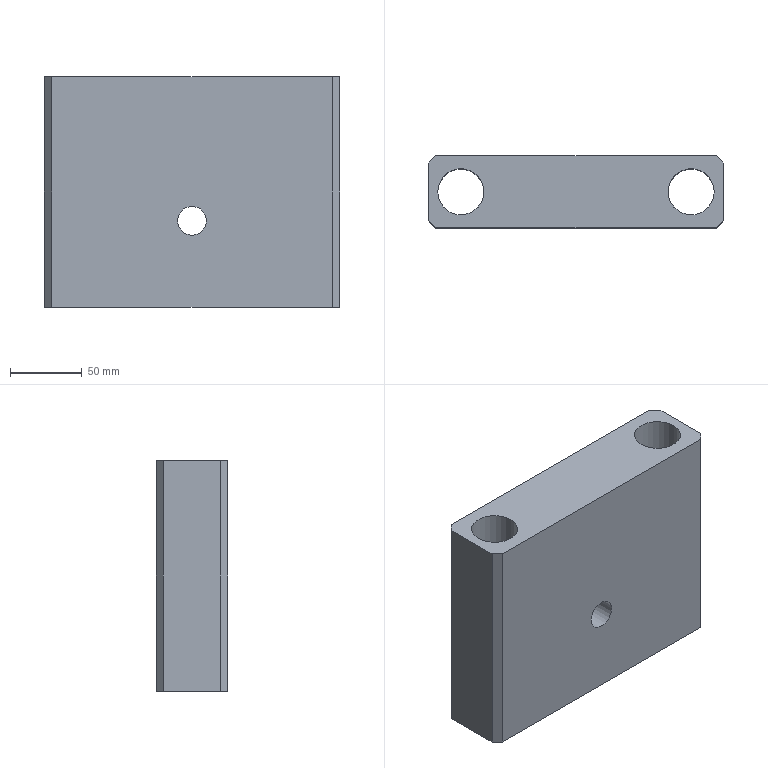Part | NX | features 001 2 | 1 solid | 22 faces | box 205 x 50 x 160 mm | volume 1357581 mm3 | plane 10 | cylinder 7 | cone 5 | commonest cylinder face diameters 5 x4 32 x2 20 x1
STEP:
#1=CARTESIAN_POINT('',(60.,8.,-311.627));
#2=VERTEX_POINT('',#1);
#3=VERTEX_LOOP('',#2);
#4=FACE_BOUND('',#3,.T.);
#5=CARTESIAN_POINT('',(60.,5.5,-313.129));
#6=VERTEX_POINT('',#5);
#7=CARTESIAN_POINT('',(60.,8.,-313.129));
#8=DIRECTION('',(0.,0.,-1.));
#9=DIRECTION('',(0.,-1.,0.));
#10=AXIS2_PLACEMENT_3D('',#7,#8,#9);
#11=CIRCLE('',#10,2.5);
#12=EDGE_CURVE('',#6,#6,#11,.T.);
#13=ORIENTED_EDGE('',*,*,#12,.T.);
#14=EDGE_LOOP('',(#13));
#15=FACE_BOUND('',#14,.T.);
#16=CARTESIAN_POINT('',(60.,8.,-311.627));
#17=DIRECTION('',(0.,0.,-1.));
#18=DIRECTION('',(0.,-1.,0.));
#19=AXIS2_PLACEMENT_3D('',#16,#17,#18);
#20=CONICAL_SURFACE('',#19,0.,1.03);
#21=ADVANCED_FACE('',(#4,#15),#20,.F.);
#22=ORIENTED_EDGE('',*,*,#12,.F.);
#23=EDGE_LOOP('',(#22));
#24=FACE_BOUND('',#23,.T.);
#25=CARTESIAN_POINT('',(60.,10.5,-328.129));
#26=VERTEX_POINT('',#25);
#27=CARTESIAN_POINT('',(60.,8.,-328.129));
#28=DIRECTION('',(0.,0.,1.));
#29=DIRECTION('',(0.,1.,0.));
#30=AXIS2_PLACEMENT_3D('',#27,#28,#29);
#31=CIRCLE('',#30,2.5);
#32=EDGE_CURVE('',#26,#26,#31,.T.);
#33=ORIENTED_EDGE('',*,*,#32,.F.);
#34=EDGE_LOOP('',(#33));
#35=FACE_BOUND('',#34,.T.);
#36=CARTESIAN_POINT('',(60.,8.,-328.129));
#37=DIRECTION('',(0.,0.,-1.));
#38=DIRECTION('',(0.,-1.,0.));
#39=AXIS2_PLACEMENT_3D('',#36,#37,#38);
#40=CYLINDRICAL_SURFACE('',#39,2.5);
#41=ADVANCED_FACE('',(#24,#35),#40,.F.);
#42=CARTESIAN_POINT('',(-60.,5.5,-313.129));
#43=VERTEX_POINT('',#42);
#44=CARTESIAN_POINT('',(-60.,8.,-313.129));
#45=DIRECTION('',(0.,0.,-1.));
#46=DIRECTION('',(0.,-1.,0.));
#47=AXIS2_PLACEMENT_3D('',#44,#45,#46);
#48=CIRCLE('',#47,2.5);
#49=EDGE_CURVE('',#43,#43,#48,.T.);
#50=ORIENTED_EDGE('',*,*,#49,.T.);
#51=EDGE_LOOP('',(#50));
#52=FACE_BOUND('',#51,.T.);
#53=CARTESIAN_POINT('',(-60.,8.,-311.627));
#54=VERTEX_POINT('',#53);
#55=VERTEX_LOOP('',#54);
#56=FACE_BOUND('',#55,.T.);
#57=CARTESIAN_POINT('',(-60.,8.,-311.627));
#58=DIRECTION('',(0.,0.,-1.));
#59=DIRECTION('',(0.,-1.,0.));
#60=AXIS2_PLACEMENT_3D('',#57,#58,#59);
#61=CONICAL_SURFACE('',#60,0.,1.03);
#62=ADVANCED_FACE('',(#52,#56),#61,.F.);
#63=CARTESIAN_POINT('',(-60.,10.5,-328.129));
#64=VERTEX_POINT('',#63);
#65=CARTESIAN_POINT('',(-60.,8.,-328.129));
#66=DIRECTION('',(0.,0.,1.));
#67=DIRECTION('',(0.,1.,0.));
#68=AXIS2_PLACEMENT_3D('',#65,#66,#67);
#69=CIRCLE('',#68,2.5);
#70=EDGE_CURVE('',#64,#64,#69,.T.);
#71=ORIENTED_EDGE('',*,*,#70,.F.);
#72=EDGE_LOOP('',(#71));
#73=FACE_BOUND('',#72,.T.);
#74=ORIENTED_EDGE('',*,*,#49,.F.);
#75=EDGE_LOOP('',(#74));
#76=FACE_BOUND('',#75,.T.);
#77=CARTESIAN_POINT('',(-60.,8.,-328.129));
#78=DIRECTION('',(0.,0.,-1.));
#79=DIRECTION('',(0.,-1.,0.));
#80=AXIS2_PLACEMENT_3D('',#77,#78,#79);
#81=CYLINDRICAL_SURFACE('',#80,2.5);
#82=ADVANCED_FACE('',(#73,#76),#81,.F.);
#83=CARTESIAN_POINT('',(-60.,39.5,-313.129));
#84=VERTEX_POINT('',#83);
#85=CARTESIAN_POINT('',(-60.,42.,-313.129));
#86=DIRECTION('',(0.,0.,-1.));
#87=DIRECTION('',(0.,-1.,0.));
#88=AXIS2_PLACEMENT_3D('',#85,#86,#87);
#89=CIRCLE('',#88,2.5);
#90=EDGE_CURVE('',#84,#84,#89,.T.);
#91=ORIENTED_EDGE('',*,*,#90,.T.);
#92=EDGE_LOOP('',(#91));
#93=FACE_BOUND('',#92,.T.);
#94=CARTESIAN_POINT('',(-60.,42.,-311.627));
#95=VERTEX_POINT('',#94);
#96=VERTEX_LOOP('',#95);
#97=FACE_BOUND('',#96,.T.);
#98=CARTESIAN_POINT('',(-60.,42.,-311.627));
#99=DIRECTION('',(0.,0.,-1.));
#100=DIRECTION('',(0.,-1.,0.));
#101=AXIS2_PLACEMENT_3D('',#98,#99,#100);
#102=CONICAL_SURFACE('',#101,0.,1.03);
#103=ADVANCED_FACE('',(#93,#97),#102,.F.);
#104=ORIENTED_EDGE('',*,*,#90,.F.);
#105=EDGE_LOOP('',(#104));
#106=FACE_BOUND('',#105,.T.);
#107=CARTESIAN_POINT('',(-60.,44.5,-328.129));
#108=VERTEX_POINT('',#107);
#109=CARTESIAN_POINT('',(-60.,42.,-328.129));
#110=DIRECTION('',(0.,0.,1.));
#111=DIRECTION('',(0.,1.,0.));
#112=AXIS2_PLACEMENT_3D('',#109,#110,#111);
#113=CIRCLE('',#112,2.5);
#114=EDGE_CURVE('',#108,#108,#113,.T.);
#115=ORIENTED_EDGE('',*,*,#114,.F.);
#116=EDGE_LOOP('',(#115));
#117=FACE_BOUND('',#116,.T.);
#118=CARTESIAN_POINT('',(-60.,42.,-328.129));
#119=DIRECTION('',(0.,0.,-1.));
#120=DIRECTION('',(0.,-1.,0.));
#121=AXIS2_PLACEMENT_3D('',#118,#119,#120);
#122=CYLINDRICAL_SURFACE('',#121,2.5);
#123=ADVANCED_FACE('',(#106,#117),#122,.F.);
#124=CARTESIAN_POINT('',(96.,25.,-328.129));
#125=VERTEX_POINT('',#124);
#126=CARTESIAN_POINT('',(80.,25.,-328.129));
#127=DIRECTION('',(0.,0.,1.));
#128=DIRECTION('',(1.,0.,0.));
#129=AXIS2_PLACEMENT_3D('',#126,#127,#128);
#130=CIRCLE('',#129,16.);
#131=EDGE_CURVE('',#125,#125,#130,.T.);
#132=ORIENTED_EDGE('',*,*,#131,.F.);
#133=EDGE_LOOP('',(#132));
#134=FACE_BOUND('',#133,.T.);
#135=CARTESIAN_POINT('',(64.,25.,-168.129));
#136=VERTEX_POINT('',#135);
#137=CARTESIAN_POINT('',(80.,25.,-168.129));
#138=DIRECTION('',(0.,0.,-1.));
#139=DIRECTION('',(-1.,0.,0.));
#140=AXIS2_PLACEMENT_3D('',#137,#138,#139);
#141=CIRCLE('',#140,16.);
#142=EDGE_CURVE('',#136,#136,#141,.T.);
#143=ORIENTED_EDGE('',*,*,#142,.F.);
#144=EDGE_LOOP('',(#143));
#145=FACE_BOUND('',#144,.T.);
#146=CARTESIAN_POINT('',(80.,25.,-328.129));
#147=DIRECTION('',(0.,0.,1.));
#148=DIRECTION('',(1.,0.,0.));
#149=AXIS2_PLACEMENT_3D('',#146,#147,#148);
#150=CYLINDRICAL_SURFACE('',#149,16.);
#151=ADVANCED_FACE('',(#134,#145),#150,.F.);
#152=CARTESIAN_POINT('',(-64.,25.,-328.129));
#153=VERTEX_POINT('',#152);
#154=CARTESIAN_POINT('',(-80.,25.,-328.129));
#155=DIRECTION('',(0.,0.,1.));
#156=DIRECTION('',(1.,0.,0.));
#157=AXIS2_PLACEMENT_3D('',#154,#155,#156);
#158=CIRCLE('',#157,16.);
#159=EDGE_CURVE('',#153,#153,#158,.T.);
#160=ORIENTED_EDGE('',*,*,#159,.F.);
#161=EDGE_LOOP('',(#160));
#162=FACE_BOUND('',#161,.T.);
#163=CARTESIAN_POINT('',(-96.,25.,-168.129));
#164=VERTEX_POINT('',#163);
#165=CARTESIAN_POINT('',(-80.,25.,-168.129));
#166=DIRECTION('',(0.,0.,-1.));
#167=DIRECTION('',(-1.,0.,0.));
#168=AXIS2_PLACEMENT_3D('',#165,#166,#167);
#169=CIRCLE('',#168,16.);
#170=EDGE_CURVE('',#164,#164,#169,.T.);
#171=ORIENTED_EDGE('',*,*,#170,.F.);
#172=EDGE_LOOP('',(#171));
#173=FACE_BOUND('',#172,.T.);
#174=CARTESIAN_POINT('',(-80.,25.,-328.129));
#175=DIRECTION('',(0.,0.,1.));
#176=DIRECTION('',(1.,0.,0.));
#177=AXIS2_PLACEMENT_3D('',#174,#175,#176);
#178=CYLINDRICAL_SURFACE('',#177,16.);
#179=ADVANCED_FACE('',(#162,#173),#178,.F.);
#180=CARTESIAN_POINT('',(102.5,45.,-168.129));
#181=VERTEX_POINT('',#180);
#182=CARTESIAN_POINT('',(102.5,45.,-328.129));
#183=VERTEX_POINT('',#182);
#184=CARTESIAN_POINT('',(102.5,45.,-168.129));
#185=DIRECTION('',(0.,0.,-1.));
#186=VECTOR('',#185,1000.);
#187=LINE('',#184,#186);
#188=EDGE_CURVE('',#181,#183,#187,.T.);
#189=ORIENTED_EDGE('',*,*,#188,.T.);
#190=CARTESIAN_POINT('',(97.5,50.,-328.129));
#191=VERTEX_POINT('',#190);
#192=CARTESIAN_POINT('',(97.5,50.,-328.129));
#193=DIRECTION('',(0.7071,-0.7071,0.));
#194=VECTOR('',#193,1000.);
#195=LINE('',#192,#194);
#196=EDGE_CURVE('',#191,#183,#195,.T.);
#197=ORIENTED_EDGE('',*,*,#196,.F.);
#198=CARTESIAN_POINT('',(97.5,50.,-168.129));
#199=VERTEX_POINT('',#198);
#200=CARTESIAN_POINT('',(97.5,50.,-328.129));
#201=DIRECTION('',(0.,0.,1.));
#202=VECTOR('',#201,1000.);
#203=LINE('',#200,#202);
#204=EDGE_CURVE('',#191,#199,#203,.T.);
#205=ORIENTED_EDGE('',*,*,#204,.T.);
#206=CARTESIAN_POINT('',(102.5,45.,-168.129));
#207=DIRECTION('',(-0.7071,0.7071,0.));
#208=VECTOR('',#207,1000.);
#209=LINE('',#206,#208);
#210=EDGE_CURVE('',#181,#199,#209,.T.);
#211=ORIENTED_EDGE('',*,*,#210,.F.);
#212=EDGE_LOOP('',(#189,#197,#205,#211));
#213=FACE_BOUND('',#212,.T.);
#214=CARTESIAN_POINT('',(97.5,50.,-248.129));
#215=DIRECTION('',(0.7071,0.7071,0.));
#216=DIRECTION('',(0.,0.,1.));
#217=AXIS2_PLACEMENT_3D('',#214,#215,#216);
#218=PLANE('',#217);
#219=ADVANCED_FACE('',(#213),#218,.T.);
#220=CARTESIAN_POINT('',(10.,48.,-268.129));
#221=VERTEX_POINT('',#220);
#222=CARTESIAN_POINT('',(0.,48.,-268.129));
#223=DIRECTION('',(0.,-1.,0.));
#224=DIRECTION('',(1.,0.,0.));
#225=AXIS2_PLACEMENT_3D('',#222,#223,#224);
#226=CIRCLE('',#225,10.);
#227=EDGE_CURVE('',#221,#221,#226,.T.);
#228=ORIENTED_EDGE('',*,*,#227,.T.);
#229=EDGE_LOOP('',(#228));
#230=FACE_BOUND('',#229,.T.);
#231=CARTESIAN_POINT('',(-12.,50.,-268.129));
#232=VERTEX_POINT('',#231);
#233=CARTESIAN_POINT('',(0.,50.,-268.129));
#234=DIRECTION('',(0.,-1.,0.));
#235=DIRECTION('',(-1.,0.,0.));
#236=AXIS2_PLACEMENT_3D('',#233,#234,#235);
#237=CIRCLE('',#236,12.);
#238=EDGE_CURVE('',#232,#232,#237,.T.);
#239=ORIENTED_EDGE('',*,*,#238,.F.);
#240=EDGE_LOOP('',(#239));
#241=FACE_BOUND('',#240,.T.);
#242=CARTESIAN_POINT('',(0.,47.775,-268.129));
#243=DIRECTION('',(0.,1.,0.));
#244=DIRECTION('',(-1.,0.,0.));
#245=AXIS2_PLACEMENT_3D('',#242,#243,#244);
#246=CONICAL_SURFACE('',#245,9.775,0.7854);
#247=ADVANCED_FACE('',(#230,#241),#246,.F.);
#248=ORIENTED_EDGE('',*,*,#227,.F.);
#249=EDGE_LOOP('',(#248));
#250=FACE_BOUND('',#249,.T.);
#251=CARTESIAN_POINT('',(-10.,0.,-268.129));
#252=VERTEX_POINT('',#251);
#253=CARTESIAN_POINT('',(0.,0.,-268.129));
#254=DIRECTION('',(0.,1.,0.));
#255=DIRECTION('',(-1.,0.,0.));
#256=AXIS2_PLACEMENT_3D('',#253,#254,#255);
#257=CIRCLE('',#256,10.);
#258=EDGE_CURVE('',#252,#252,#257,.T.);
#259=ORIENTED_EDGE('',*,*,#258,.F.);
#260=EDGE_LOOP('',(#259));
#261=FACE_BOUND('',#260,.T.);
#262=CARTESIAN_POINT('',(0.,0.,-268.129));
#263=DIRECTION('',(0.,1.,0.));
#264=DIRECTION('',(-1.,0.,0.));
#265=AXIS2_PLACEMENT_3D('',#262,#263,#264);
#266=CYLINDRICAL_SURFACE('',#265,10.);
#267=ADVANCED_FACE('',(#250,#261),#266,.F.);
#268=CARTESIAN_POINT('',(-102.5,45.,-328.129));
#269=VERTEX_POINT('',#268);
#270=CARTESIAN_POINT('',(-102.5,45.,-168.129));
#271=VERTEX_POINT('',#270);
#272=CARTESIAN_POINT('',(-102.5,45.,-328.129));
#273=DIRECTION('',(0.,0.,1.));
#274=VECTOR('',#273,1000.);
#275=LINE('',#272,#274);
#276=EDGE_CURVE('',#269,#271,#275,.T.);
#277=ORIENTED_EDGE('',*,*,#276,.T.);
#278=CARTESIAN_POINT('',(-97.5,50.,-168.129));
#279=VERTEX_POINT('',#278);
#280=CARTESIAN_POINT('',(-97.5,50.,-168.129));
#281=DIRECTION('',(-0.7071,-0.7071,0.));
#282=VECTOR('',#281,1000.);
#283=LINE('',#280,#282);
#284=EDGE_CURVE('',#279,#271,#283,.T.);
#285=ORIENTED_EDGE('',*,*,#284,.F.);
#286=CARTESIAN_POINT('',(-97.5,50.,-328.129));
#287=VERTEX_POINT('',#286);
#288=CARTESIAN_POINT('',(-97.5,50.,-168.129));
#289=DIRECTION('',(0.,0.,-1.));
#290=VECTOR('',#289,1000.);
#291=LINE('',#288,#290);
#292=EDGE_CURVE('',#279,#287,#291,.T.);
#293=ORIENTED_EDGE('',*,*,#292,.T.);
#294=CARTESIAN_POINT('',(-102.5,45.,-328.129));
#295=DIRECTION('',(0.7071,0.7071,0.));
#296=VECTOR('',#295,1000.);
#297=LINE('',#294,#296);
#298=EDGE_CURVE('',#269,#287,#297,.T.);
#299=ORIENTED_EDGE('',*,*,#298,.F.);
#300=EDGE_LOOP('',(#277,#285,#293,#299));
#301=FACE_BOUND('',#300,.T.);
#302=CARTESIAN_POINT('',(-97.5,50.,-248.129));
#303=DIRECTION('',(-0.7071,0.7071,0.));
#304=DIRECTION('',(0.,0.,-1.));
#305=AXIS2_PLACEMENT_3D('',#302,#303,#304);
#306=PLANE('',#305);
#307=ADVANCED_FACE('',(#301),#306,.T.);
#308=ORIENTED_EDGE('',*,*,#276,.F.);
#309=CARTESIAN_POINT('',(-102.5,5.,-328.129));
#310=VERTEX_POINT('',#309);
#311=CARTESIAN_POINT('',(-102.5,5.,-328.129));
#312=DIRECTION('',(0.,1.,0.));
#313=VECTOR('',#312,1000.);
#314=LINE('',#311,#313);
#315=EDGE_CURVE('',#310,#269,#314,.T.);
#316=ORIENTED_EDGE('',*,*,#315,.F.);
#317=CARTESIAN_POINT('',(-102.5,5.,-168.129));
#318=VERTEX_POINT('',#317);
#319=CARTESIAN_POINT('',(-102.5,5.,-168.129));
#320=DIRECTION('',(0.,0.,-1.));
#321=VECTOR('',#320,1000.);
#322=LINE('',#319,#321);
#323=EDGE_CURVE('',#318,#310,#322,.T.);
#324=ORIENTED_EDGE('',*,*,#323,.F.);
#325=CARTESIAN_POINT('',(-102.5,5.,-168.129));
#326=DIRECTION('',(0.,1.,0.));
#327=VECTOR('',#326,1000.);
#328=LINE('',#325,#327);
#329=EDGE_CURVE('',#318,#271,#328,.T.);
#330=ORIENTED_EDGE('',*,*,#329,.T.);
#331=EDGE_LOOP('',(#308,#316,#324,#330));
#332=FACE_BOUND('',#331,.T.);
#333=CARTESIAN_POINT('',(-102.5,50.,-328.129));
#334=DIRECTION('',(1.,0.,0.));
#335=DIRECTION('',(0.,1.,0.));
#336=AXIS2_PLACEMENT_3D('',#333,#334,#335);
#337=PLANE('',#336);
#338=ADVANCED_FACE('',(#332),#337,.F.);
#339=CARTESIAN_POINT('',(-97.5,0.,-328.129));
#340=VERTEX_POINT('',#339);
#341=CARTESIAN_POINT('',(-97.5,0.,-168.129));
#342=VERTEX_POINT('',#341);
#343=CARTESIAN_POINT('',(-97.5,0.,-328.129));
#344=DIRECTION('',(0.,0.,1.));
#345=VECTOR('',#344,1000.);
#346=LINE('',#343,#345);
#347=EDGE_CURVE('',#340,#342,#346,.T.);
#348=ORIENTED_EDGE('',*,*,#347,.T.);
#349=CARTESIAN_POINT('',(-102.5,5.,-168.129));
#350=DIRECTION('',(0.7071,-0.7071,0.));
#351=VECTOR('',#350,1000.);
#352=LINE('',#349,#351);
#353=EDGE_CURVE('',#318,#342,#352,.T.);
#354=ORIENTED_EDGE('',*,*,#353,.F.);
#355=ORIENTED_EDGE('',*,*,#323,.T.);
#356=CARTESIAN_POINT('',(-97.5,0.,-328.129));
#357=DIRECTION('',(-0.7071,0.7071,0.));
#358=VECTOR('',#357,1000.);
#359=LINE('',#356,#358);
#360=EDGE_CURVE('',#340,#310,#359,.T.);
#361=ORIENTED_EDGE('',*,*,#360,.F.);
#362=EDGE_LOOP('',(#348,#354,#355,#361));
#363=FACE_BOUND('',#362,.T.);
#364=CARTESIAN_POINT('',(-102.5,5.,-328.129));
#365=DIRECTION('',(0.7071,0.7071,0.));
#366=DIRECTION('',(0.,0.,1.));
#367=AXIS2_PLACEMENT_3D('',#364,#365,#366);
#368=PLANE('',#367);
#369=ADVANCED_FACE('',(#363),#368,.F.);
#370=ORIENTED_EDGE('',*,*,#258,.T.);
#371=EDGE_LOOP('',(#370));
#372=FACE_BOUND('',#371,.T.);
#373=ORIENTED_EDGE('',*,*,#347,.F.);
#374=CARTESIAN_POINT('',(97.5,0.,-328.129));
#375=VERTEX_POINT('',#374);
#376=CARTESIAN_POINT('',(-97.5,0.,-328.129));
#377=DIRECTION('',(1.,0.,0.));
#378=VECTOR('',#377,1000.);
#379=LINE('',#376,#378);
#380=EDGE_CURVE('',#340,#375,#379,.T.);
#381=ORIENTED_EDGE('',*,*,#380,.T.);
#382=CARTESIAN_POINT('',(97.5,0.,-168.129));
#383=VERTEX_POINT('',#382);
#384=CARTESIAN_POINT('',(97.5,0.,-168.129));
#385=DIRECTION('',(0.,0.,-1.));
#386=VECTOR('',#385,1000.);
#387=LINE('',#384,#386);
#388=EDGE_CURVE('',#383,#375,#387,.T.);
#389=ORIENTED_EDGE('',*,*,#388,.F.);
#390=CARTESIAN_POINT('',(97.5,0.,-168.129));
#391=DIRECTION('',(-1.,0.,0.));
#392=VECTOR('',#391,1000.);
#393=LINE('',#390,#392);
#394=EDGE_CURVE('',#383,#342,#393,.T.);
#395=ORIENTED_EDGE('',*,*,#394,.T.);
#396=EDGE_LOOP('',(#373,#381,#389,#395));
#397=FACE_BOUND('',#396,.T.);
#398=CARTESIAN_POINT('',(0.,0.,-248.129));
#399=DIRECTION('',(0.,1.,0.));
#400=DIRECTION('',(-1.,0.,0.));
#401=AXIS2_PLACEMENT_3D('',#398,#399,#400);
#402=PLANE('',#401);
#403=ADVANCED_FACE('',(#372,#397),#402,.F.);
#404=ORIENTED_EDGE('',*,*,#388,.T.);
#405=CARTESIAN_POINT('',(102.5,5.,-328.129));
#406=VERTEX_POINT('',#405);
#407=CARTESIAN_POINT('',(102.5,5.,-328.129));
#408=DIRECTION('',(-0.7071,-0.7071,0.));
#409=VECTOR('',#408,1000.);
#410=LINE('',#407,#409);
#411=EDGE_CURVE('',#406,#375,#410,.T.);
#412=ORIENTED_EDGE('',*,*,#411,.F.);
#413=CARTESIAN_POINT('',(102.5,5.,-168.129));
#414=VERTEX_POINT('',#413);
#415=CARTESIAN_POINT('',(102.5,5.,-328.129));
#416=DIRECTION('',(0.,0.,1.));
#417=VECTOR('',#416,1000.);
#418=LINE('',#415,#417);
#419=EDGE_CURVE('',#406,#414,#418,.T.);
#420=ORIENTED_EDGE('',*,*,#419,.T.);
#421=CARTESIAN_POINT('',(97.5,0.,-168.129));
#422=DIRECTION('',(0.7071,0.7071,0.));
#423=VECTOR('',#422,1000.);
#424=LINE('',#421,#423);
#425=EDGE_CURVE('',#383,#414,#424,.T.);
#426=ORIENTED_EDGE('',*,*,#425,.F.);
#427=EDGE_LOOP('',(#404,#412,#420,#426));
#428=FACE_BOUND('',#427,.T.);
#429=CARTESIAN_POINT('',(102.5,5.,-328.129));
#430=DIRECTION('',(-0.7071,0.7071,0.));
#431=DIRECTION('',(0.,0.,-1.));
#432=AXIS2_PLACEMENT_3D('',#429,#430,#431);
#433=PLANE('',#432);
#434=ADVANCED_FACE('',(#428),#433,.F.);
#435=ORIENTED_EDGE('',*,*,#188,.F.);
#436=CARTESIAN_POINT('',(102.5,5.,-168.129));
#437=DIRECTION('',(0.,1.,0.));
#438=VECTOR('',#437,1000.);
#439=LINE('',#436,#438);
#440=EDGE_CURVE('',#414,#181,#439,.T.);
#441=ORIENTED_EDGE('',*,*,#440,.F.);
#442=ORIENTED_EDGE('',*,*,#419,.F.);
#443=CARTESIAN_POINT('',(102.5,5.,-328.129));
#444=DIRECTION('',(0.,1.,0.));
#445=VECTOR('',#444,1000.);
#446=LINE('',#443,#445);
#447=EDGE_CURVE('',#406,#183,#446,.T.);
#448=ORIENTED_EDGE('',*,*,#447,.T.);
#449=EDGE_LOOP('',(#435,#441,#442,#448));
#450=FACE_BOUND('',#449,.T.);
#451=CARTESIAN_POINT('',(102.5,50.,-328.129));
#452=DIRECTION('',(-1.,0.,0.));
#453=DIRECTION('',(0.,-1.,0.));
#454=AXIS2_PLACEMENT_3D('',#451,#452,#453);
#455=PLANE('',#454);
#456=ADVANCED_FACE('',(#450),#455,.F.);
#457=ORIENTED_EDGE('',*,*,#142,.T.);
#458=EDGE_LOOP('',(#457));
#459=FACE_BOUND('',#458,.T.);
#460=ORIENTED_EDGE('',*,*,#170,.T.);
#461=EDGE_LOOP('',(#460));
#462=FACE_BOUND('',#461,.T.);
#463=ORIENTED_EDGE('',*,*,#210,.T.);
#464=CARTESIAN_POINT('',(97.5,50.,-168.129));
#465=DIRECTION('',(-1.,0.,0.));
#466=VECTOR('',#465,1000.);
#467=LINE('',#464,#466);
#468=EDGE_CURVE('',#199,#279,#467,.T.);
#469=ORIENTED_EDGE('',*,*,#468,.T.);
#470=ORIENTED_EDGE('',*,*,#284,.T.);
#471=ORIENTED_EDGE('',*,*,#329,.F.);
#472=ORIENTED_EDGE('',*,*,#353,.T.);
#473=ORIENTED_EDGE('',*,*,#394,.F.);
#474=ORIENTED_EDGE('',*,*,#425,.T.);
#475=ORIENTED_EDGE('',*,*,#440,.T.);
#476=EDGE_LOOP('',(#463,#469,#470,#471,#472,#473,#474,#475));
#477=FACE_BOUND('',#476,.T.);
#478=CARTESIAN_POINT('',(-102.5,50.,-168.129));
#479=DIRECTION('',(0.,0.,-1.));
#480=DIRECTION('',(-1.,0.,0.));
#481=AXIS2_PLACEMENT_3D('',#478,#479,#480);
#482=PLANE('',#481);
#483=ADVANCED_FACE('',(#459,#462,#477),#482,.F.);
#484=ORIENTED_EDGE('',*,*,#238,.T.);
#485=EDGE_LOOP('',(#484));
#486=FACE_BOUND('',#485,.T.);
#487=ORIENTED_EDGE('',*,*,#204,.F.);
#488=CARTESIAN_POINT('',(-97.5,50.,-328.129));
#489=DIRECTION('',(1.,0.,0.));
#490=VECTOR('',#489,1000.);
#491=LINE('',#488,#490);
#492=EDGE_CURVE('',#287,#191,#491,.T.);
#493=ORIENTED_EDGE('',*,*,#492,.F.);
#494=ORIENTED_EDGE('',*,*,#292,.F.);
#495=ORIENTED_EDGE('',*,*,#468,.F.);
#496=EDGE_LOOP('',(#487,#493,#494,#495));
#497=FACE_BOUND('',#496,.T.);
#498=CARTESIAN_POINT('',(0.,50.,-248.129));
#499=DIRECTION('',(0.,1.,0.));
#500=DIRECTION('',(-1.,0.,0.));
#501=AXIS2_PLACEMENT_3D('',#498,#499,#500);
#502=PLANE('',#501);
#503=ADVANCED_FACE('',(#486,#497),#502,.T.);
#504=ORIENTED_EDGE('',*,*,#131,.T.);
#505=EDGE_LOOP('',(#504));
#506=FACE_BOUND('',#505,.T.);
#507=ORIENTED_EDGE('',*,*,#159,.T.);
#508=EDGE_LOOP('',(#507));
#509=FACE_BOUND('',#508,.T.);
#510=ORIENTED_EDGE('',*,*,#32,.T.);
#511=EDGE_LOOP('',(#510));
#512=FACE_BOUND('',#511,.T.);
#513=ORIENTED_EDGE('',*,*,#70,.T.);
#514=EDGE_LOOP('',(#513));
#515=FACE_BOUND('',#514,.T.);
#516=ORIENTED_EDGE('',*,*,#114,.T.);
#517=EDGE_LOOP('',(#516));
#518=FACE_BOUND('',#517,.T.);
#519=CARTESIAN_POINT('',(60.,39.5,-328.129));
#520=VERTEX_POINT('',#519);
#521=CARTESIAN_POINT('',(60.,42.,-328.129));
#522=DIRECTION('',(0.,0.,1.));
#523=DIRECTION('',(0.,-1.,0.));
#524=AXIS2_PLACEMENT_3D('',#521,#522,#523);
#525=CIRCLE('',#524,2.5);
#526=EDGE_CURVE('',#520,#520,#525,.T.);
#527=ORIENTED_EDGE('',*,*,#526,.T.);
#528=EDGE_LOOP('',(#527));
#529=FACE_BOUND('',#528,.T.);
#530=ORIENTED_EDGE('',*,*,#196,.T.);
#531=ORIENTED_EDGE('',*,*,#447,.F.);
#532=ORIENTED_EDGE('',*,*,#411,.T.);
#533=ORIENTED_EDGE('',*,*,#380,.F.);
#534=ORIENTED_EDGE('',*,*,#360,.T.);
#535=ORIENTED_EDGE('',*,*,#315,.T.);
#536=ORIENTED_EDGE('',*,*,#298,.T.);
#537=ORIENTED_EDGE('',*,*,#492,.T.);
#538=EDGE_LOOP('',(#530,#531,#532,#533,#534,#535,#536,#537));
#539=FACE_BOUND('',#538,.T.);
#540=CARTESIAN_POINT('',(-102.5,50.,-328.129));
#541=DIRECTION('',(0.,0.,1.));
#542=DIRECTION('',(1.,0.,0.));
#543=AXIS2_PLACEMENT_3D('',#540,#541,#542);
#544=PLANE('',#543);
#545=ADVANCED_FACE('',(#506,#509,#512,#515,#518,#529,#539),#544,.F.);
#546=CARTESIAN_POINT('',(60.,42.,-311.627));
#547=VERTEX_POINT('',#546);
#548=VERTEX_LOOP('',#547);
#549=FACE_BOUND('',#548,.T.);
#550=CARTESIAN_POINT('',(60.,44.5,-313.129));
#551=VERTEX_POINT('',#550);
#552=CARTESIAN_POINT('',(60.,42.,-313.129));
#553=DIRECTION('',(0.,0.,-1.));
#554=DIRECTION('',(0.,1.,0.));
#555=AXIS2_PLACEMENT_3D('',#552,#553,#554);
#556=CIRCLE('',#555,2.5);
#557=EDGE_CURVE('',#551,#551,#556,.T.);
#558=ORIENTED_EDGE('',*,*,#557,.T.);
#559=EDGE_LOOP('',(#558));
#560=FACE_BOUND('',#559,.T.);
#561=CARTESIAN_POINT('',(60.,42.,-311.627));
#562=DIRECTION('',(0.,0.,-1.));
#563=DIRECTION('',(0.,-1.,0.));
#564=AXIS2_PLACEMENT_3D('',#561,#562,#563);
#565=CONICAL_SURFACE('',#564,0.,1.03);
#566=ADVANCED_FACE('',(#549,#560),#565,.F.);
#567=ORIENTED_EDGE('',*,*,#557,.F.);
#568=EDGE_LOOP('',(#567));
#569=FACE_BOUND('',#568,.T.);
#570=ORIENTED_EDGE('',*,*,#526,.F.);
#571=EDGE_LOOP('',(#570));
#572=FACE_BOUND('',#571,.T.);
#573=CARTESIAN_POINT('',(60.,42.,-328.129));
#574=DIRECTION('',(0.,0.,-1.));
#575=DIRECTION('',(0.,-1.,0.));
#576=AXIS2_PLACEMENT_3D('',#573,#574,#575);
#577=CYLINDRICAL_SURFACE('',#576,2.5);
#578=ADVANCED_FACE('',(#569,#572),#577,.F.);
#579=CLOSED_SHELL('',(#21,#41,#62,#82,#103,#123,#151,#179,#219,#247,#267,#307,#338,#369,#403,#434,#456,#483,#503,#545,#566,#578));
#580=MANIFOLD_SOLID_BREP('',#579);
#581=(LENGTH_UNIT()NAMED_UNIT(*)SI_UNIT(.MILLI.,.METRE.));
#582=UNCERTAINTY_MEASURE_WITH_UNIT(LENGTH_MEASURE(0.00001),#581,'','');
#583=(NAMED_UNIT(*)PLANE_ANGLE_UNIT()SI_UNIT($,.RADIAN.));
#584=(NAMED_UNIT(*)SI_UNIT($,.STERADIAN.)SOLID_ANGLE_UNIT());
#585=(GEOMETRIC_REPRESENTATION_CONTEXT(3)GLOBAL_UNCERTAINTY_ASSIGNED_CONTEXT((#582))GLOBAL_UNIT_ASSIGNED_CONTEXT((#581,#583,#584))REPRESENTATION_CONTEXT('',''));
#586=ADVANCED_BREP_SHAPE_REPRESENTATION('',(#580),#585);